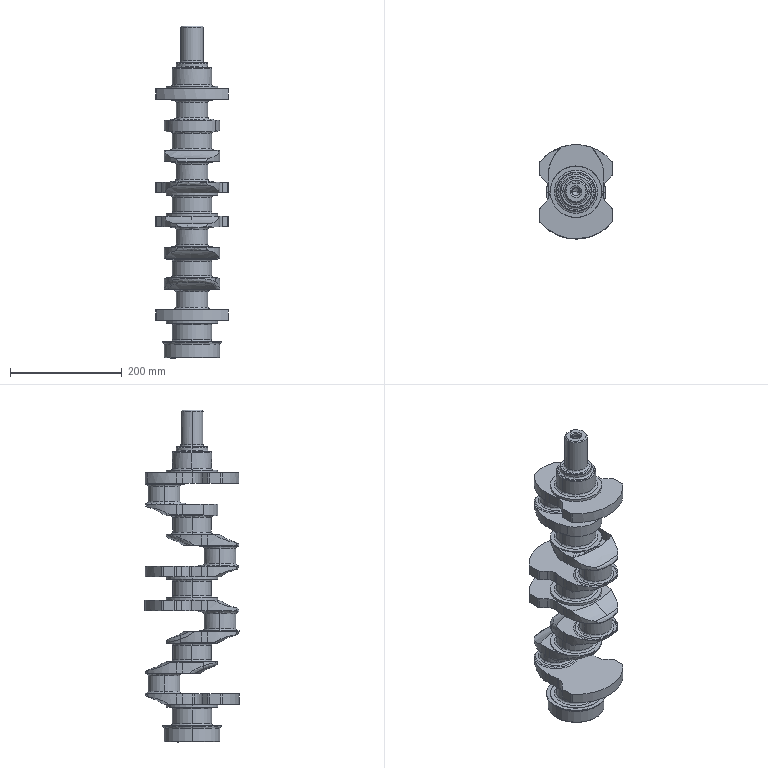Part | SolidWorks | features BaseBody 1 | 1 solid | 360 faces | box 130 x 168.108 x 593 mm | volume 3326856 mm3 | cylinder 147 | spline 92 | plane 74 | cone 47 | commonest cylinder face diameters 92 x22 40 x17 10 x16 140 x16 170 x16 11 x12